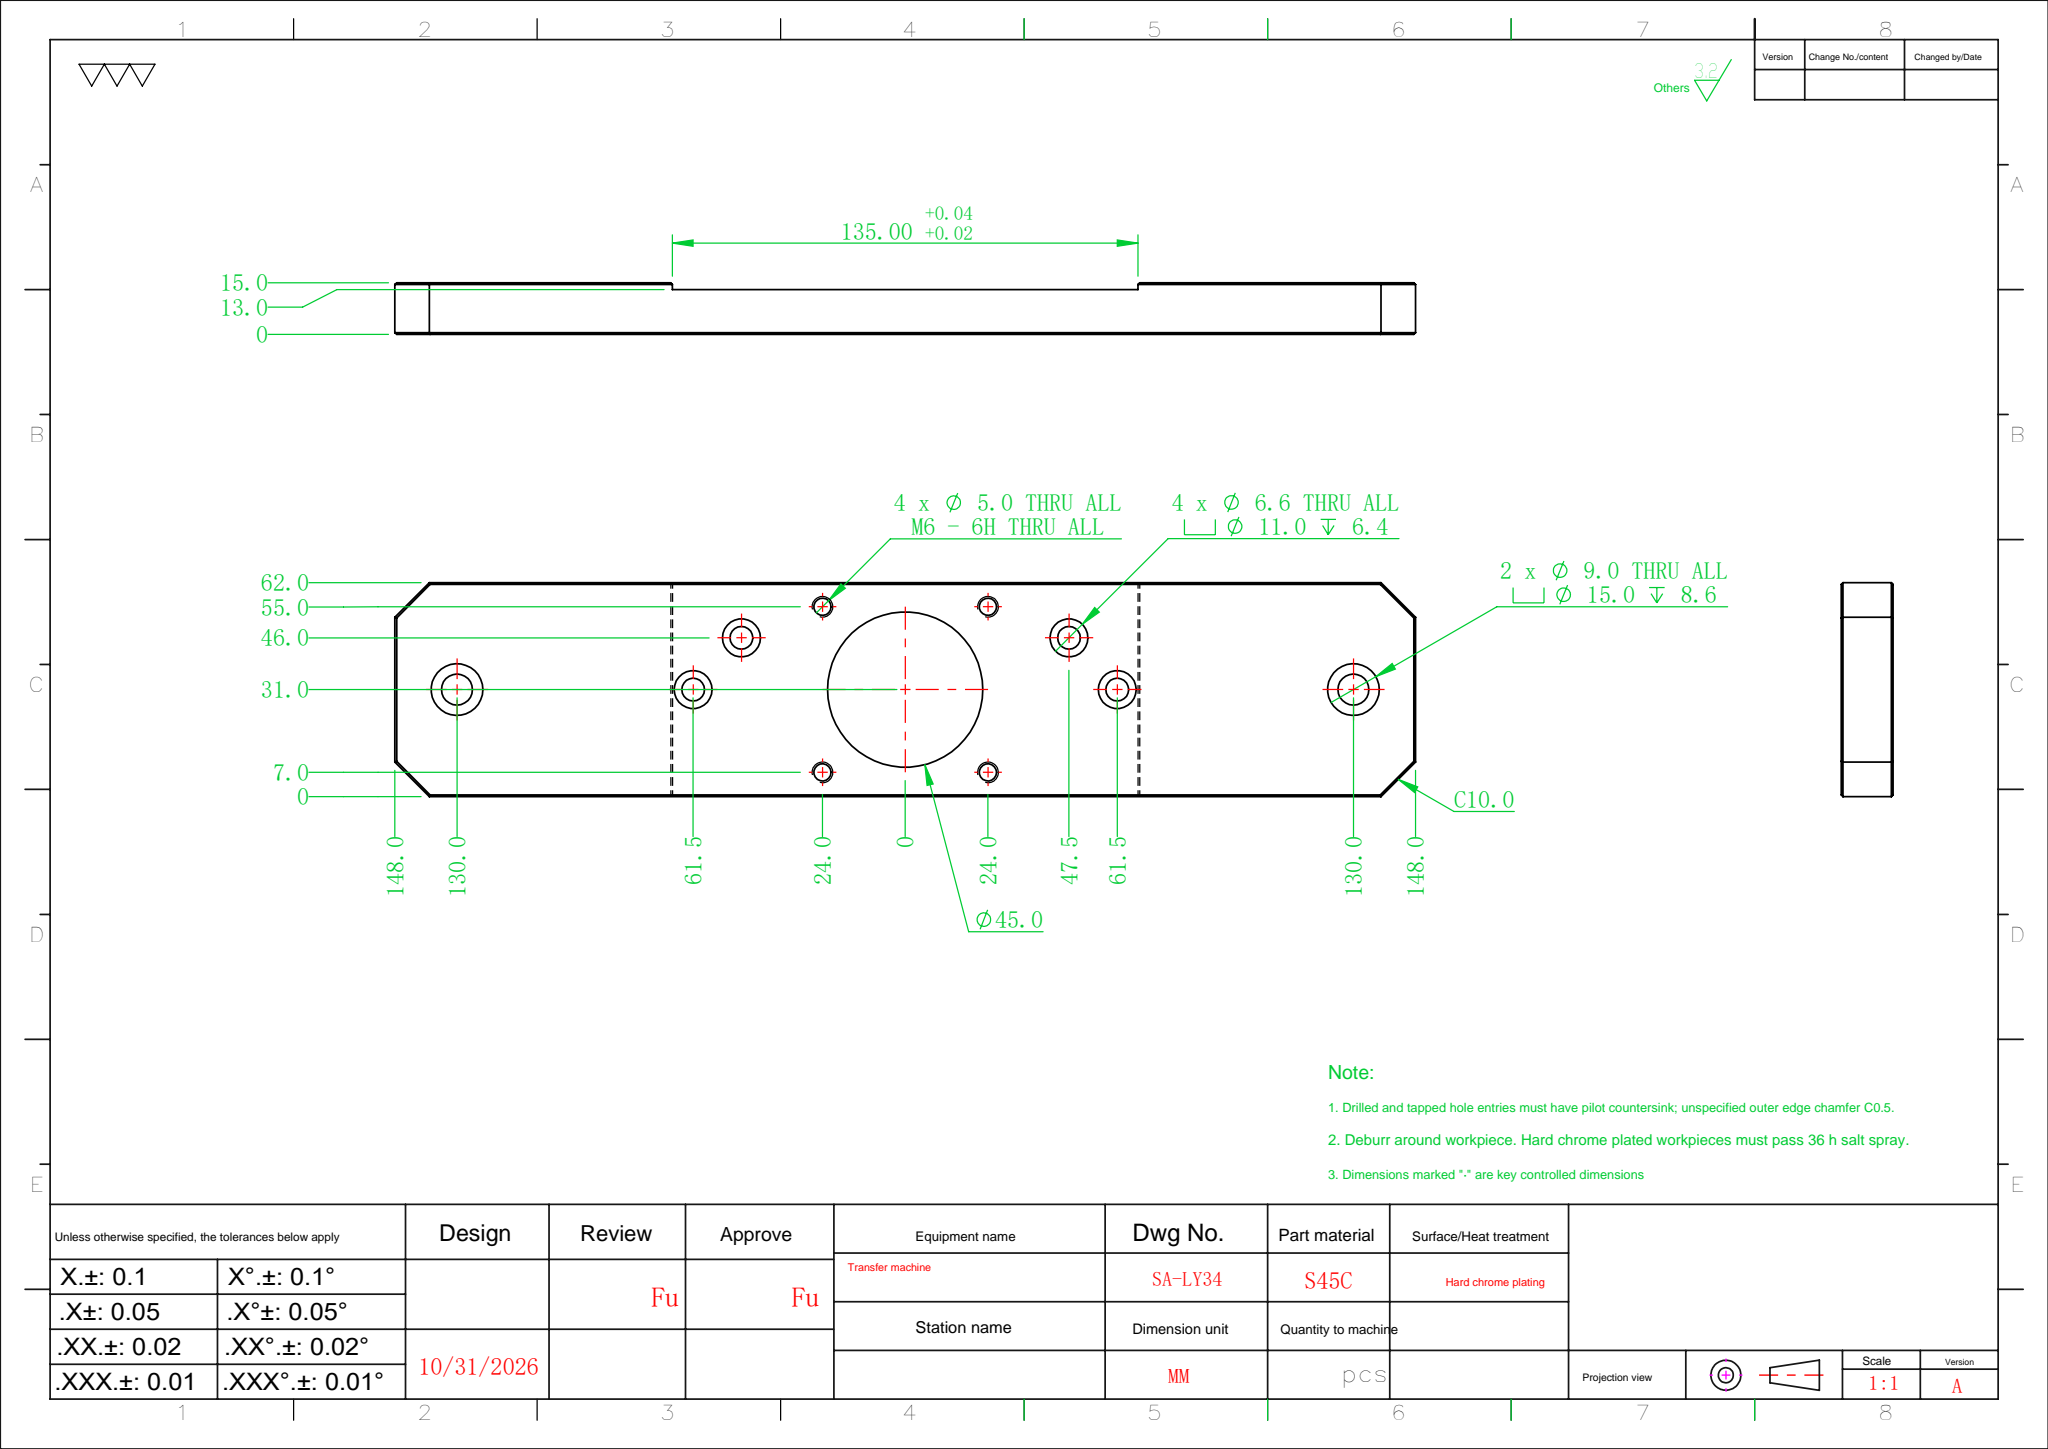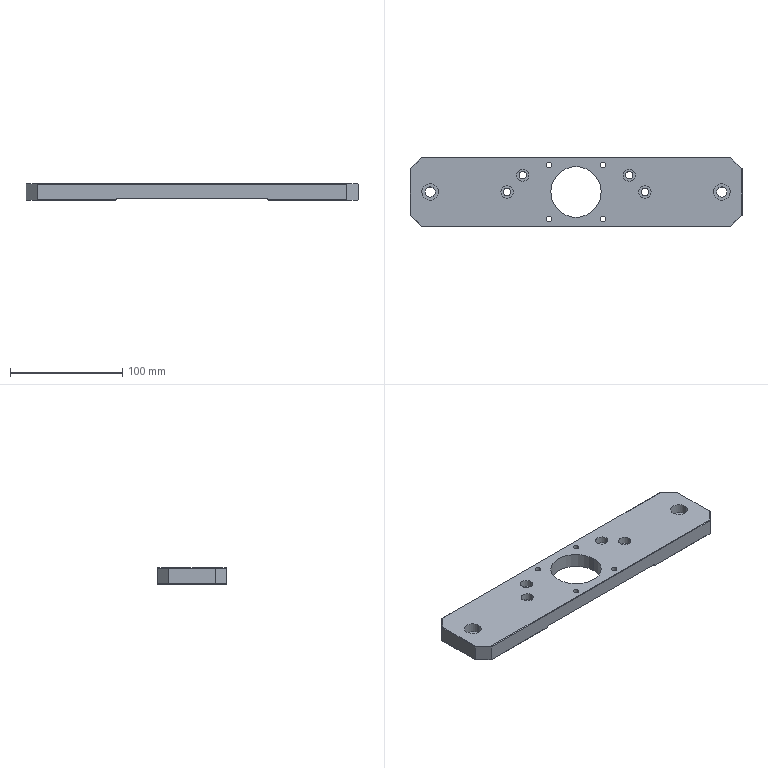Part | SolidWorks | features HoleWzd 3, Chamfer 2, Cut 2, Extrusion 1 | 1 solid | 74 faces | box 296 x 62 x 15 mm | volume 226499 mm3 | plane 40 | cylinder 34 | commonest cylinder face diameters 5 x8 6.6 x8 11 x8 9 x4 15 x4 45 x2